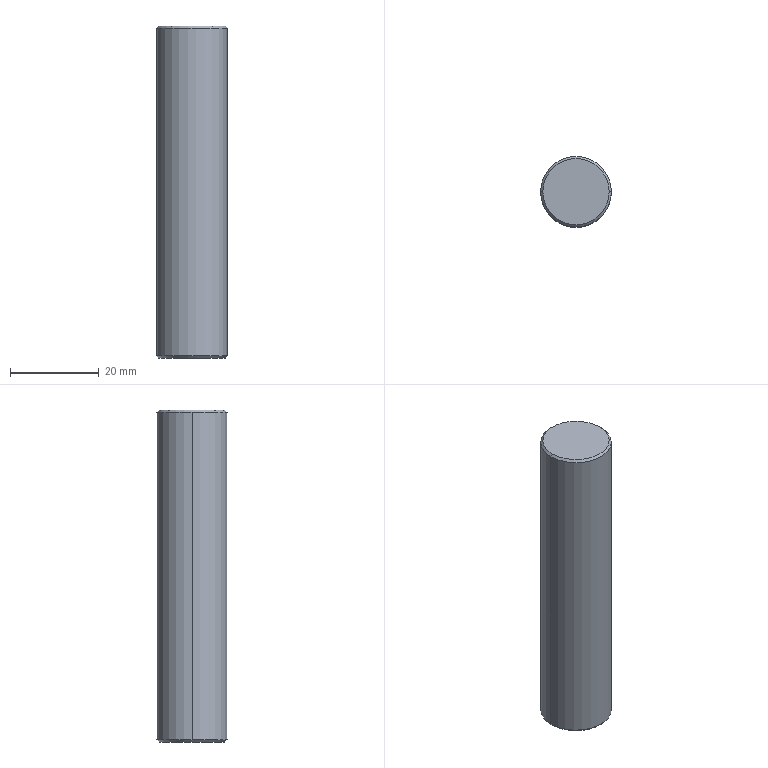Part | NX | features BREP 1 | 1 solid | 8 faces | box 16 x 16 x 75 mm | volume 15067 mm3 | cone 4 | cylinder 2 | plane 2 | commonest cylinder face diameters 16 x2
STEP:
#1=CARTESIAN_POINT('',(7.5,0.,75.));
#2=VERTEX_POINT('',#1);
#3=CARTESIAN_POINT('',(-7.5,0.,75.));
#4=VERTEX_POINT('',#3);
#5=CARTESIAN_POINT('',(0.,0.,75.));
#6=DIRECTION('',(0.,0.,1.));
#7=DIRECTION('',(1.,0.,0.));
#8=AXIS2_PLACEMENT_3D('',#5,#6,#7);
#9=CIRCLE('',#8,7.5);
#10=EDGE_CURVE('',#2,#4,#9,.T.);
#11=ORIENTED_EDGE('',*,*,#10,.F.);
#12=CARTESIAN_POINT('',(8.,0.,74.5));
#13=VERTEX_POINT('',#12);
#14=CARTESIAN_POINT('',(7.5,0.,75.));
#15=DIRECTION('',(0.7071,0.,-0.7071));
#16=VECTOR('',#15,1000.);
#17=LINE('',#14,#16);
#18=EDGE_CURVE('',#2,#13,#17,.T.);
#19=ORIENTED_EDGE('',*,*,#18,.T.);
#20=CARTESIAN_POINT('',(-8.,0.,74.5));
#21=VERTEX_POINT('',#20);
#22=CARTESIAN_POINT('',(0.,0.,74.5));
#23=DIRECTION('',(0.,0.,-1.));
#24=DIRECTION('',(1.,0.,0.));
#25=AXIS2_PLACEMENT_3D('',#22,#23,#24);
#26=CIRCLE('',#25,8.);
#27=EDGE_CURVE('',#21,#13,#26,.T.);
#28=ORIENTED_EDGE('',*,*,#27,.F.);
#29=CARTESIAN_POINT('',(-7.5,0.,75.));
#30=DIRECTION('',(-0.7071,0.,-0.7071));
#31=VECTOR('',#30,1000.);
#32=LINE('',#29,#31);
#33=EDGE_CURVE('',#4,#21,#32,.T.);
#34=ORIENTED_EDGE('',*,*,#33,.F.);
#35=EDGE_LOOP('',(#11,#19,#28,#34));
#36=FACE_BOUND('',#35,.T.);
#37=CARTESIAN_POINT('',(0.,0.,75.));
#38=DIRECTION('',(0.,0.,-1.));
#39=DIRECTION('',(-1.,0.,0.));
#40=AXIS2_PLACEMENT_3D('',#37,#38,#39);
#41=CONICAL_SURFACE('',#40,7.5,0.7854);
#42=ADVANCED_FACE('',(#36),#41,.T.);
#43=CARTESIAN_POINT('',(-7.5,0.,0.));
#44=VERTEX_POINT('',#43);
#45=CARTESIAN_POINT('',(7.5,0.,0.));
#46=VERTEX_POINT('',#45);
#47=CARTESIAN_POINT('',(0.,0.,0.));
#48=DIRECTION('',(0.,0.,-1.));
#49=DIRECTION('',(1.,0.,0.));
#50=AXIS2_PLACEMENT_3D('',#47,#48,#49);
#51=CIRCLE('',#50,7.5);
#52=EDGE_CURVE('',#44,#46,#51,.T.);
#53=ORIENTED_EDGE('',*,*,#52,.F.);
#54=CARTESIAN_POINT('',(-8.,0.,0.5));
#55=VERTEX_POINT('',#54);
#56=CARTESIAN_POINT('',(-8.,0.,0.5));
#57=DIRECTION('',(-0.7071,0.,0.7071));
#58=VECTOR('',#57,1000.);
#59=LINE('',#56,#58);
#60=EDGE_CURVE('',#55,#44,#59,.F.);
#61=ORIENTED_EDGE('',*,*,#60,.F.);
#62=CARTESIAN_POINT('',(8.,0.,0.5));
#63=VERTEX_POINT('',#62);
#64=CARTESIAN_POINT('',(0.,0.,0.5));
#65=DIRECTION('',(0.,0.,1.));
#66=DIRECTION('',(1.,0.,0.));
#67=AXIS2_PLACEMENT_3D('',#64,#65,#66);
#68=CIRCLE('',#67,8.);
#69=EDGE_CURVE('',#63,#55,#68,.T.);
#70=ORIENTED_EDGE('',*,*,#69,.F.);
#71=CARTESIAN_POINT('',(8.,0.,0.5));
#72=DIRECTION('',(0.7071,0.,0.7071));
#73=VECTOR('',#72,1000.);
#74=LINE('',#71,#73);
#75=EDGE_CURVE('',#63,#46,#74,.F.);
#76=ORIENTED_EDGE('',*,*,#75,.T.);
#77=EDGE_LOOP('',(#53,#61,#70,#76));
#78=FACE_BOUND('',#77,.T.);
#79=CARTESIAN_POINT('',(0.,0.,0.5));
#80=DIRECTION('',(0.,0.,1.));
#81=DIRECTION('',(1.,0.,0.));
#82=AXIS2_PLACEMENT_3D('',#79,#80,#81);
#83=CONICAL_SURFACE('',#82,8.,0.7854);
#84=ADVANCED_FACE('',(#78),#83,.T.);
#85=ORIENTED_EDGE('',*,*,#27,.T.);
#86=CARTESIAN_POINT('',(8.,0.,75.));
#87=DIRECTION('',(0.,0.,-1.));
#88=VECTOR('',#87,1000.);
#89=LINE('',#86,#88);
#90=EDGE_CURVE('',#13,#63,#89,.T.);
#91=ORIENTED_EDGE('',*,*,#90,.T.);
#92=ORIENTED_EDGE('',*,*,#69,.T.);
#93=CARTESIAN_POINT('',(-8.,0.,75.));
#94=DIRECTION('',(0.,0.,-1.));
#95=VECTOR('',#94,1000.);
#96=LINE('',#93,#95);
#97=EDGE_CURVE('',#21,#55,#96,.T.);
#98=ORIENTED_EDGE('',*,*,#97,.F.);
#99=EDGE_LOOP('',(#85,#91,#92,#98));
#100=FACE_BOUND('',#99,.T.);
#101=CARTESIAN_POINT('',(0.,0.,75.));
#102=DIRECTION('',(0.,0.,-1.));
#103=DIRECTION('',(-1.,0.,0.));
#104=AXIS2_PLACEMENT_3D('',#101,#102,#103);
#105=CYLINDRICAL_SURFACE('',#104,8.);
#106=ADVANCED_FACE('',(#100),#105,.T.);
#107=ORIENTED_EDGE('',*,*,#90,.F.);
#108=CARTESIAN_POINT('',(0.,0.,74.5));
#109=DIRECTION('',(0.,0.,-1.));
#110=DIRECTION('',(1.,0.,0.));
#111=AXIS2_PLACEMENT_3D('',#108,#109,#110);
#112=CIRCLE('',#111,8.);
#113=EDGE_CURVE('',#13,#21,#112,.T.);
#114=ORIENTED_EDGE('',*,*,#113,.T.);
#115=ORIENTED_EDGE('',*,*,#97,.T.);
#116=CARTESIAN_POINT('',(0.,0.,0.5));
#117=DIRECTION('',(0.,0.,1.));
#118=DIRECTION('',(1.,0.,0.));
#119=AXIS2_PLACEMENT_3D('',#116,#117,#118);
#120=CIRCLE('',#119,8.);
#121=EDGE_CURVE('',#55,#63,#120,.T.);
#122=ORIENTED_EDGE('',*,*,#121,.T.);
#123=EDGE_LOOP('',(#107,#114,#115,#122));
#124=FACE_BOUND('',#123,.T.);
#125=CARTESIAN_POINT('',(0.,0.,75.));
#126=DIRECTION('',(0.,0.,-1.));
#127=DIRECTION('',(-1.,0.,0.));
#128=AXIS2_PLACEMENT_3D('',#125,#126,#127);
#129=CYLINDRICAL_SURFACE('',#128,8.);
#130=ADVANCED_FACE('',(#124),#129,.T.);
#131=CARTESIAN_POINT('',(0.,0.,75.));
#132=DIRECTION('',(0.,0.,1.));
#133=DIRECTION('',(1.,0.,0.));
#134=AXIS2_PLACEMENT_3D('',#131,#132,#133);
#135=CIRCLE('',#134,7.5);
#136=EDGE_CURVE('',#4,#2,#135,.T.);
#137=ORIENTED_EDGE('',*,*,#136,.T.);
#138=ORIENTED_EDGE('',*,*,#10,.T.);
#139=EDGE_LOOP('',(#137,#138));
#140=FACE_BOUND('',#139,.T.);
#141=CARTESIAN_POINT('',(0.,0.,75.));
#142=DIRECTION('',(0.,0.,1.));
#143=DIRECTION('',(1.,0.,0.));
#144=AXIS2_PLACEMENT_3D('',#141,#142,#143);
#145=PLANE('',#144);
#146=ADVANCED_FACE('',(#140),#145,.T.);
#147=CARTESIAN_POINT('',(0.,0.,0.));
#148=DIRECTION('',(0.,0.,-1.));
#149=DIRECTION('',(1.,0.,0.));
#150=AXIS2_PLACEMENT_3D('',#147,#148,#149);
#151=CIRCLE('',#150,7.5);
#152=EDGE_CURVE('',#46,#44,#151,.T.);
#153=ORIENTED_EDGE('',*,*,#152,.T.);
#154=ORIENTED_EDGE('',*,*,#52,.T.);
#155=EDGE_LOOP('',(#153,#154));
#156=FACE_BOUND('',#155,.T.);
#157=CARTESIAN_POINT('',(0.,0.,0.));
#158=DIRECTION('',(0.,0.,1.));
#159=DIRECTION('',(1.,0.,0.));
#160=AXIS2_PLACEMENT_3D('',#157,#158,#159);
#161=PLANE('',#160);
#162=ADVANCED_FACE('',(#156),#161,.F.);
#163=ORIENTED_EDGE('',*,*,#60,.T.);
#164=ORIENTED_EDGE('',*,*,#152,.F.);
#165=ORIENTED_EDGE('',*,*,#75,.F.);
#166=ORIENTED_EDGE('',*,*,#121,.F.);
#167=EDGE_LOOP('',(#163,#164,#165,#166));
#168=FACE_BOUND('',#167,.T.);
#169=CARTESIAN_POINT('',(0.,0.,0.5));
#170=DIRECTION('',(0.,0.,1.));
#171=DIRECTION('',(1.,0.,0.));
#172=AXIS2_PLACEMENT_3D('',#169,#170,#171);
#173=CONICAL_SURFACE('',#172,8.,0.7854);
#174=ADVANCED_FACE('',(#168),#173,.T.);
#175=ORIENTED_EDGE('',*,*,#18,.F.);
#176=ORIENTED_EDGE('',*,*,#136,.F.);
#177=ORIENTED_EDGE('',*,*,#33,.T.);
#178=ORIENTED_EDGE('',*,*,#113,.F.);
#179=EDGE_LOOP('',(#175,#176,#177,#178));
#180=FACE_BOUND('',#179,.T.);
#181=CARTESIAN_POINT('',(0.,0.,75.));
#182=DIRECTION('',(0.,0.,-1.));
#183=DIRECTION('',(-1.,0.,0.));
#184=AXIS2_PLACEMENT_3D('',#181,#182,#183);
#185=CONICAL_SURFACE('',#184,7.5,0.7854);
#186=ADVANCED_FACE('',(#180),#185,.T.);
#187=CLOSED_SHELL('',(#42,#84,#106,#130,#146,#162,#174,#186));
#188=MANIFOLD_SOLID_BREP('',#187);
#189=(LENGTH_UNIT()NAMED_UNIT(*)SI_UNIT(.MILLI.,.METRE.));
#190=UNCERTAINTY_MEASURE_WITH_UNIT(LENGTH_MEASURE(0.00001),#189,'','');
#191=(NAMED_UNIT(*)PLANE_ANGLE_UNIT()SI_UNIT($,.RADIAN.));
#192=(NAMED_UNIT(*)SI_UNIT($,.STERADIAN.)SOLID_ANGLE_UNIT());
#193=(GEOMETRIC_REPRESENTATION_CONTEXT(3)GLOBAL_UNCERTAINTY_ASSIGNED_CONTEXT((#190))GLOBAL_UNIT_ASSIGNED_CONTEXT((#189,#191,#192))REPRESENTATION_CONTEXT('',''));
#194=ADVANCED_BREP_SHAPE_REPRESENTATION('',(#188),#193);